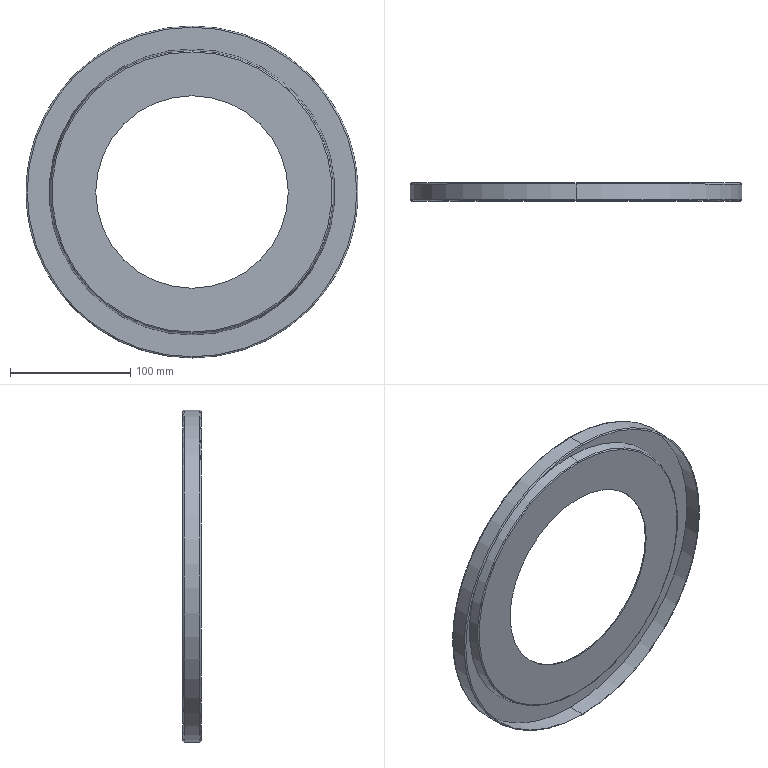Part | SolidWorks | features ICE 2, Fillet 1, Revolution 1 | 1 solid | 25 faces | box 276 x 15 x 276 mm | volume 56604 mm3 | cylinder 8 | torus 8 | plane 5 | cone 4 | commonest cylinder face diameters 160 x2 230 x2 274 x2 276 x2
STEP:
#1=CARTESIAN_POINT('',(0.,-1.,-80.));
#2=VERTEX_POINT('',#1);
#3=CARTESIAN_POINT('',(0.,-1.,80.));
#4=VERTEX_POINT('',#3);
#5=CARTESIAN_POINT('',(0.,-1.,0.));
#6=DIRECTION('',(0.,1.,0.));
#7=DIRECTION('',(0.,0.,1.));
#8=AXIS2_PLACEMENT_3D('',#5,#6,#7);
#9=CIRCLE('',#8,80.);
#10=EDGE_CURVE('',#2,#4,#9,.T.);
#11=ORIENTED_EDGE('',*,*,#10,.F.);
#12=CARTESIAN_POINT('',(0.,-0.01,-80.));
#13=VERTEX_POINT('',#12);
#14=CARTESIAN_POINT('',(0.,-6.,-80.));
#15=DIRECTION('',(0.,1.,0.));
#16=VECTOR('',#15,1000.);
#17=LINE('',#14,#16);
#18=EDGE_CURVE('',#2,#13,#17,.T.);
#19=ORIENTED_EDGE('',*,*,#18,.T.);
#20=CARTESIAN_POINT('',(0.,-0.01,80.));
#21=VERTEX_POINT('',#20);
#22=CARTESIAN_POINT('',(0.,-0.01,0.));
#23=DIRECTION('',(0.,1.,0.));
#24=DIRECTION('',(0.,0.,1.));
#25=AXIS2_PLACEMENT_3D('',#22,#23,#24);
#26=CIRCLE('',#25,80.);
#27=EDGE_CURVE('',#13,#21,#26,.T.);
#28=ORIENTED_EDGE('',*,*,#27,.T.);
#29=CARTESIAN_POINT('',(0.,-6.,80.));
#30=DIRECTION('',(0.,1.,0.));
#31=VECTOR('',#30,1000.);
#32=LINE('',#29,#31);
#33=EDGE_CURVE('',#4,#21,#32,.T.);
#34=ORIENTED_EDGE('',*,*,#33,.F.);
#35=EDGE_LOOP('',(#11,#19,#28,#34));
#36=FACE_OUTER_BOUND('',#35,.T.);
#37=CARTESIAN_POINT('',(0.,-6.,0.));
#38=DIRECTION('',(0.,1.,0.));
#39=DIRECTION('',(0.,0.,1.));
#40=AXIS2_PLACEMENT_3D('',#37,#38,#39);
#41=CYLINDRICAL_SURFACE('',#40,80.);
#42=ADVANCED_FACE('',(#36),#41,.F.);
#43=CARTESIAN_POINT('',(0.,9.,137.));
#44=VERTEX_POINT('',#43);
#45=CARTESIAN_POINT('',(0.,9.,-137.));
#46=VERTEX_POINT('',#45);
#47=CARTESIAN_POINT('',(0.,9.,0.));
#48=DIRECTION('',(0.,1.,0.));
#49=DIRECTION('',(0.,0.,-1.));
#50=AXIS2_PLACEMENT_3D('',#47,#48,#49);
#51=CIRCLE('',#50,137.);
#52=EDGE_CURVE('',#44,#46,#51,.T.);
#53=ORIENTED_EDGE('',*,*,#52,.F.);
#54=CARTESIAN_POINT('',(0.,8.,138.));
#55=VERTEX_POINT('',#54);
#56=CARTESIAN_POINT('',(0.,8.,137.));
#57=DIRECTION('',(1.,0.,0.));
#58=DIRECTION('',(0.,0.,-1.));
#59=AXIS2_PLACEMENT_3D('',#56,#57,#58);
#60=CIRCLE('',#59,1.);
#61=EDGE_CURVE('',#44,#55,#60,.T.);
#62=ORIENTED_EDGE('',*,*,#61,.T.);
#63=CARTESIAN_POINT('',(0.,8.,-138.));
#64=VERTEX_POINT('',#63);
#65=CARTESIAN_POINT('',(0.,8.,0.));
#66=DIRECTION('',(0.,-1.,0.));
#67=DIRECTION('',(0.,0.,-1.));
#68=AXIS2_PLACEMENT_3D('',#65,#66,#67);
#69=CIRCLE('',#68,138.);
#70=EDGE_CURVE('',#64,#55,#69,.T.);
#71=ORIENTED_EDGE('',*,*,#70,.F.);
#72=CARTESIAN_POINT('',(0.,8.,-137.));
#73=DIRECTION('',(-1.,0.,0.));
#74=DIRECTION('',(0.,0.,1.));
#75=AXIS2_PLACEMENT_3D('',#72,#73,#74);
#76=CIRCLE('',#75,1.);
#77=EDGE_CURVE('',#46,#64,#76,.T.);
#78=ORIENTED_EDGE('',*,*,#77,.F.);
#79=EDGE_LOOP('',(#53,#62,#71,#78));
#80=FACE_OUTER_BOUND('',#79,.T.);
#81=CARTESIAN_POINT('',(0.,8.,0.));
#82=DIRECTION('',(0.,-1.,0.));
#83=DIRECTION('',(0.,0.,-1.));
#84=AXIS2_PLACEMENT_3D('',#81,#82,#83);
#85=TOROIDAL_SURFACE('',#84,137.,1.);
#86=ADVANCED_FACE('',(#80),#85,.T.);
#87=CARTESIAN_POINT('',(0.,8.174,117.854));
#88=VERTEX_POINT('',#87);
#89=CARTESIAN_POINT('',(0.,8.174,-117.854));
#90=VERTEX_POINT('',#89);
#91=CARTESIAN_POINT('',(0.,8.174,0.));
#92=DIRECTION('',(0.,1.,0.));
#93=DIRECTION('',(0.,0.,-1.));
#94=AXIS2_PLACEMENT_3D('',#91,#92,#93);
#95=CIRCLE('',#94,117.854);
#96=EDGE_CURVE('',#88,#90,#95,.T.);
#97=ORIENTED_EDGE('',*,*,#96,.F.);
#98=CARTESIAN_POINT('',(0.,9.,118.839));
#99=VERTEX_POINT('',#98);
#100=CARTESIAN_POINT('',(0.,8.,118.839));
#101=DIRECTION('',(1.,0.,0.));
#102=DIRECTION('',(0.,0.,-1.));
#103=AXIS2_PLACEMENT_3D('',#100,#101,#102);
#104=CIRCLE('',#103,1.);
#105=EDGE_CURVE('',#88,#99,#104,.T.);
#106=ORIENTED_EDGE('',*,*,#105,.T.);
#107=CARTESIAN_POINT('',(0.,9.,-118.839));
#108=VERTEX_POINT('',#107);
#109=CARTESIAN_POINT('',(0.,9.,0.));
#110=DIRECTION('',(0.,-1.,0.));
#111=DIRECTION('',(0.,0.,-1.));
#112=AXIS2_PLACEMENT_3D('',#109,#110,#111);
#113=CIRCLE('',#112,118.839);
#114=EDGE_CURVE('',#108,#99,#113,.T.);
#115=ORIENTED_EDGE('',*,*,#114,.F.);
#116=CARTESIAN_POINT('',(0.,8.,-118.839));
#117=DIRECTION('',(-1.,0.,0.));
#118=DIRECTION('',(0.,0.,1.));
#119=AXIS2_PLACEMENT_3D('',#116,#117,#118);
#120=CIRCLE('',#119,1.);
#121=EDGE_CURVE('',#90,#108,#120,.T.);
#122=ORIENTED_EDGE('',*,*,#121,.F.);
#123=EDGE_LOOP('',(#97,#106,#115,#122));
#124=FACE_OUTER_BOUND('',#123,.T.);
#125=CARTESIAN_POINT('',(0.,8.,0.));
#126=DIRECTION('',(0.,-1.,0.));
#127=DIRECTION('',(0.,0.,-1.));
#128=AXIS2_PLACEMENT_3D('',#125,#126,#127);
#129=TOROIDAL_SURFACE('',#128,118.839,1.);
#130=ADVANCED_FACE('',(#124),#129,.T.);
#131=CARTESIAN_POINT('',(0.,-6.,-137.));
#132=VERTEX_POINT('',#131);
#133=CARTESIAN_POINT('',(0.,-6.,137.));
#134=VERTEX_POINT('',#133);
#135=CARTESIAN_POINT('',(0.,-6.,0.));
#136=DIRECTION('',(0.,-1.,0.));
#137=DIRECTION('',(0.,0.,-1.));
#138=AXIS2_PLACEMENT_3D('',#135,#136,#137);
#139=CIRCLE('',#138,137.);
#140=EDGE_CURVE('',#132,#134,#139,.T.);
#141=ORIENTED_EDGE('',*,*,#140,.F.);
#142=CARTESIAN_POINT('',(0.,-5.,-138.));
#143=VERTEX_POINT('',#142);
#144=CARTESIAN_POINT('',(0.,-5.,-137.));
#145=DIRECTION('',(1.,0.,0.));
#146=DIRECTION('',(0.,0.,-1.));
#147=AXIS2_PLACEMENT_3D('',#144,#145,#146);
#148=CIRCLE('',#147,1.);
#149=EDGE_CURVE('',#132,#143,#148,.T.);
#150=ORIENTED_EDGE('',*,*,#149,.T.);
#151=CARTESIAN_POINT('',(0.,-5.,138.));
#152=VERTEX_POINT('',#151);
#153=CARTESIAN_POINT('',(0.,-5.,0.));
#154=DIRECTION('',(0.,1.,0.));
#155=DIRECTION('',(0.,0.,1.));
#156=AXIS2_PLACEMENT_3D('',#153,#154,#155);
#157=CIRCLE('',#156,138.);
#158=EDGE_CURVE('',#152,#143,#157,.T.);
#159=ORIENTED_EDGE('',*,*,#158,.F.);
#160=CARTESIAN_POINT('',(0.,-5.,137.));
#161=DIRECTION('',(-1.,0.,0.));
#162=DIRECTION('',(0.,0.,1.));
#163=AXIS2_PLACEMENT_3D('',#160,#161,#162);
#164=CIRCLE('',#163,1.);
#165=EDGE_CURVE('',#134,#152,#164,.T.);
#166=ORIENTED_EDGE('',*,*,#165,.F.);
#167=EDGE_LOOP('',(#141,#150,#159,#166));
#168=FACE_OUTER_BOUND('',#167,.T.);
#169=CARTESIAN_POINT('',(0.,-5.,0.));
#170=DIRECTION('',(0.,1.,0.));
#171=DIRECTION('',(0.,0.,1.));
#172=AXIS2_PLACEMENT_3D('',#169,#170,#171);
#173=TOROIDAL_SURFACE('',#172,137.,1.);
#174=ADVANCED_FACE('',(#168),#173,.T.);
#175=CARTESIAN_POINT('',(0.,-1.,-116.413));
#176=VERTEX_POINT('',#175);
#177=CARTESIAN_POINT('',(0.,-1.,116.413));
#178=VERTEX_POINT('',#177);
#179=CARTESIAN_POINT('',(0.,-1.,0.));
#180=DIRECTION('',(0.,-1.,0.));
#181=DIRECTION('',(0.,0.,1.));
#182=AXIS2_PLACEMENT_3D('',#179,#180,#181);
#183=CIRCLE('',#182,116.413);
#184=EDGE_CURVE('',#176,#178,#183,.T.);
#185=ORIENTED_EDGE('',*,*,#184,.F.);
#186=CARTESIAN_POINT('',(0.,-0.1736,-117.398));
#187=VERTEX_POINT('',#186);
#188=CARTESIAN_POINT('',(0.,0.,-116.413));
#189=DIRECTION('',(1.,0.,0.));
#190=DIRECTION('',(0.,0.,-1.));
#191=AXIS2_PLACEMENT_3D('',#188,#189,#190);
#192=CIRCLE('',#191,1.);
#193=EDGE_CURVE('',#176,#187,#192,.T.);
#194=ORIENTED_EDGE('',*,*,#193,.T.);
#195=CARTESIAN_POINT('',(0.,-0.1736,117.398));
#196=VERTEX_POINT('',#195);
#197=CARTESIAN_POINT('',(0.,-0.1736,0.));
#198=DIRECTION('',(0.,1.,0.));
#199=DIRECTION('',(0.,0.,-1.));
#200=AXIS2_PLACEMENT_3D('',#197,#198,#199);
#201=CIRCLE('',#200,117.398);
#202=EDGE_CURVE('',#196,#187,#201,.T.);
#203=ORIENTED_EDGE('',*,*,#202,.F.);
#204=CARTESIAN_POINT('',(0.,0.,116.413));
#205=DIRECTION('',(-1.,0.,0.));
#206=DIRECTION('',(0.,0.,1.));
#207=AXIS2_PLACEMENT_3D('',#204,#205,#206);
#208=CIRCLE('',#207,1.);
#209=EDGE_CURVE('',#178,#196,#208,.T.);
#210=ORIENTED_EDGE('',*,*,#209,.F.);
#211=EDGE_LOOP('',(#185,#194,#203,#210));
#212=FACE_OUTER_BOUND('',#211,.T.);
#213=CARTESIAN_POINT('',(0.,0.,0.));
#214=DIRECTION('',(0.,1.,0.));
#215=DIRECTION('',(0.,0.,1.));
#216=AXIS2_PLACEMENT_3D('',#213,#214,#215);
#217=TOROIDAL_SURFACE('',#216,116.413,1.);
#218=ADVANCED_FACE('',(#212),#217,.T.);
#219=CARTESIAN_POINT('',(0.,-0.01,-115.));
#220=VERTEX_POINT('',#219);
#221=CARTESIAN_POINT('',(0.,-0.01,115.));
#222=VERTEX_POINT('',#221);
#223=CARTESIAN_POINT('',(0.,-0.01,0.));
#224=DIRECTION('',(0.,1.,0.));
#225=DIRECTION('',(0.,0.,1.));
#226=AXIS2_PLACEMENT_3D('',#223,#224,#225);
#227=CIRCLE('',#226,115.);
#228=EDGE_CURVE('',#220,#222,#227,.T.);
#229=ORIENTED_EDGE('',*,*,#228,.F.);
#230=CARTESIAN_POINT('',(0.,0.,-115.));
#231=VERTEX_POINT('',#230);
#232=CARTESIAN_POINT('',(0.,-0.01,-115.));
#233=DIRECTION('',(0.,1.,0.));
#234=VECTOR('',#233,1000.);
#235=LINE('',#232,#234);
#236=EDGE_CURVE('',#220,#231,#235,.T.);
#237=ORIENTED_EDGE('',*,*,#236,.T.);
#238=CARTESIAN_POINT('',(0.,0.,115.));
#239=VERTEX_POINT('',#238);
#240=CARTESIAN_POINT('',(0.,0.,0.));
#241=DIRECTION('',(0.,1.,0.));
#242=DIRECTION('',(0.,0.,1.));
#243=AXIS2_PLACEMENT_3D('',#240,#241,#242);
#244=CIRCLE('',#243,115.);
#245=EDGE_CURVE('',#231,#239,#244,.T.);
#246=ORIENTED_EDGE('',*,*,#245,.T.);
#247=CARTESIAN_POINT('',(0.,-0.01,115.));
#248=DIRECTION('',(0.,1.,0.));
#249=VECTOR('',#248,1000.);
#250=LINE('',#247,#249);
#251=EDGE_CURVE('',#222,#239,#250,.T.);
#252=ORIENTED_EDGE('',*,*,#251,.F.);
#253=EDGE_LOOP('',(#229,#237,#246,#252));
#254=FACE_OUTER_BOUND('',#253,.T.);
#255=CARTESIAN_POINT('',(0.,-0.01,0.));
#256=DIRECTION('',(0.,1.,0.));
#257=DIRECTION('',(0.,0.,1.));
#258=AXIS2_PLACEMENT_3D('',#255,#256,#257);
#259=CYLINDRICAL_SURFACE('',#258,115.);
#260=ADVANCED_FACE('',(#254),#259,.F.);
#261=ORIENTED_EDGE('',*,*,#202,.T.);
#262=CARTESIAN_POINT('',(0.,8.,-118.839));
#263=VERTEX_POINT('',#262);
#264=CARTESIAN_POINT('',(0.,8.,-118.839));
#265=DIRECTION('',(0.,0.9848,-0.1736));
#266=VECTOR('',#265,1000.);
#267=LINE('',#264,#266);
#268=EDGE_CURVE('',#187,#263,#267,.T.);
#269=ORIENTED_EDGE('',*,*,#268,.T.);
#270=CARTESIAN_POINT('',(0.,8.,118.839));
#271=VERTEX_POINT('',#270);
#272=CARTESIAN_POINT('',(0.,8.,0.));
#273=DIRECTION('',(0.,-1.,0.));
#274=DIRECTION('',(0.,0.,-1.));
#275=AXIS2_PLACEMENT_3D('',#272,#273,#274);
#276=CIRCLE('',#275,118.839);
#277=EDGE_CURVE('',#263,#271,#276,.T.);
#278=ORIENTED_EDGE('',*,*,#277,.T.);
#279=CARTESIAN_POINT('',(0.,8.,118.839));
#280=DIRECTION('',(0.,0.9848,0.1736));
#281=VECTOR('',#280,1000.);
#282=LINE('',#279,#281);
#283=EDGE_CURVE('',#196,#271,#282,.T.);
#284=ORIENTED_EDGE('',*,*,#283,.F.);
#285=EDGE_LOOP('',(#261,#269,#278,#284));
#286=FACE_OUTER_BOUND('',#285,.T.);
#287=CARTESIAN_POINT('',(0.,8.,0.));
#288=DIRECTION('',(0.,1.,0.));
#289=DIRECTION('',(0.,0.,1.));
#290=AXIS2_PLACEMENT_3D('',#287,#288,#289);
#291=CONICAL_SURFACE('',#290,118.839,0.1745);
#292=ADVANCED_FACE('',(#286),#291,.T.);
#293=CARTESIAN_POINT('',(0.,8.,137.));
#294=VERTEX_POINT('',#293);
#295=CARTESIAN_POINT('',(0.,8.,-137.));
#296=VERTEX_POINT('',#295);
#297=CARTESIAN_POINT('',(0.,8.,0.));
#298=DIRECTION('',(0.,-1.,0.));
#299=DIRECTION('',(0.,0.,-1.));
#300=AXIS2_PLACEMENT_3D('',#297,#298,#299);
#301=CIRCLE('',#300,137.);
#302=EDGE_CURVE('',#294,#296,#301,.T.);
#303=ORIENTED_EDGE('',*,*,#302,.F.);
#304=CARTESIAN_POINT('',(0.,0.,137.));
#305=DIRECTION('',(0.,-1.,0.));
#306=VECTOR('',#305,1000.);
#307=LINE('',#304,#306);
#308=EDGE_CURVE('',#294,#134,#307,.T.);
#309=ORIENTED_EDGE('',*,*,#308,.T.);
#310=CARTESIAN_POINT('',(0.,-6.,0.));
#311=DIRECTION('',(0.,-1.,0.));
#312=DIRECTION('',(0.,0.,-1.));
#313=AXIS2_PLACEMENT_3D('',#310,#311,#312);
#314=CIRCLE('',#313,137.);
#315=EDGE_CURVE('',#134,#132,#314,.T.);
#316=ORIENTED_EDGE('',*,*,#315,.T.);
#317=CARTESIAN_POINT('',(0.,0.,-137.));
#318=DIRECTION('',(0.,-1.,0.));
#319=VECTOR('',#318,1000.);
#320=LINE('',#317,#319);
#321=EDGE_CURVE('',#296,#132,#320,.T.);
#322=ORIENTED_EDGE('',*,*,#321,.F.);
#323=EDGE_LOOP('',(#303,#309,#316,#322));
#324=FACE_OUTER_BOUND('',#323,.T.);
#325=CARTESIAN_POINT('',(0.,0.,0.));
#326=DIRECTION('',(0.,-1.,0.));
#327=DIRECTION('',(0.,0.,-1.));
#328=AXIS2_PLACEMENT_3D('',#325,#326,#327);
#329=CYLINDRICAL_SURFACE('',#328,137.);
#330=ADVANCED_FACE('',(#324),#329,.F.);
#331=ORIENTED_EDGE('',*,*,#70,.T.);
#332=CARTESIAN_POINT('',(0.,0.,138.));
#333=DIRECTION('',(0.,-1.,0.));
#334=VECTOR('',#333,1000.);
#335=LINE('',#332,#334);
#336=EDGE_CURVE('',#55,#152,#335,.T.);
#337=ORIENTED_EDGE('',*,*,#336,.T.);
#338=ORIENTED_EDGE('',*,*,#158,.T.);
#339=CARTESIAN_POINT('',(0.,0.,-138.));
#340=DIRECTION('',(0.,-1.,0.));
#341=VECTOR('',#340,1000.);
#342=LINE('',#339,#341);
#343=EDGE_CURVE('',#64,#143,#342,.T.);
#344=ORIENTED_EDGE('',*,*,#343,.F.);
#345=EDGE_LOOP('',(#331,#337,#338,#344));
#346=FACE_OUTER_BOUND('',#345,.T.);
#347=CARTESIAN_POINT('',(0.,0.,0.));
#348=DIRECTION('',(0.,-1.,0.));
#349=DIRECTION('',(0.,0.,-1.));
#350=AXIS2_PLACEMENT_3D('',#347,#348,#349);
#351=CYLINDRICAL_SURFACE('',#350,138.);
#352=ADVANCED_FACE('',(#346),#351,.T.);
#353=CARTESIAN_POINT('',(0.,0.,116.413));
#354=VERTEX_POINT('',#353);
#355=CARTESIAN_POINT('',(0.,0.,-116.413));
#356=VERTEX_POINT('',#355);
#357=CARTESIAN_POINT('',(0.,0.,0.));
#358=DIRECTION('',(0.,-1.,0.));
#359=DIRECTION('',(0.,0.,-1.));
#360=AXIS2_PLACEMENT_3D('',#357,#358,#359);
#361=CIRCLE('',#360,116.413);
#362=EDGE_CURVE('',#354,#356,#361,.T.);
#363=ORIENTED_EDGE('',*,*,#362,.T.);
#364=CARTESIAN_POINT('',(0.,0.,-116.413));
#365=DIRECTION('',(0.,0.9848,-0.1736));
#366=VECTOR('',#365,1000.);
#367=LINE('',#364,#366);
#368=EDGE_CURVE('',#356,#90,#367,.T.);
#369=ORIENTED_EDGE('',*,*,#368,.T.);
#370=CARTESIAN_POINT('',(0.,8.174,0.));
#371=DIRECTION('',(0.,1.,0.));
#372=DIRECTION('',(0.,0.,-1.));
#373=AXIS2_PLACEMENT_3D('',#370,#371,#372);
#374=CIRCLE('',#373,117.854);
#375=EDGE_CURVE('',#90,#88,#374,.T.);
#376=ORIENTED_EDGE('',*,*,#375,.T.);
#377=CARTESIAN_POINT('',(0.,0.,116.413));
#378=DIRECTION('',(0.,0.9848,0.1736));
#379=VECTOR('',#378,1000.);
#380=LINE('',#377,#379);
#381=EDGE_CURVE('',#354,#88,#380,.T.);
#382=ORIENTED_EDGE('',*,*,#381,.F.);
#383=EDGE_LOOP('',(#363,#369,#376,#382));
#384=FACE_OUTER_BOUND('',#383,.T.);
#385=CARTESIAN_POINT('',(0.,0.,0.));
#386=DIRECTION('',(0.,1.,0.));
#387=DIRECTION('',(0.,0.,1.));
#388=AXIS2_PLACEMENT_3D('',#385,#386,#387);
#389=CONICAL_SURFACE('',#388,116.413,0.1745);
#390=ADVANCED_FACE('',(#384),#389,.F.);
#391=CARTESIAN_POINT('',(0.,0.,0.));
#392=DIRECTION('',(0.,1.,0.));
#393=DIRECTION('',(0.,0.,1.));
#394=AXIS2_PLACEMENT_3D('',#391,#392,#393);
#395=CIRCLE('',#394,115.);
#396=EDGE_CURVE('',#239,#231,#395,.T.);
#397=ORIENTED_EDGE('',*,*,#396,.F.);
#398=ORIENTED_EDGE('',*,*,#245,.F.);
#399=EDGE_LOOP('',(#397,#398));
#400=FACE_BOUND('',#399,.T.);
#401=ORIENTED_EDGE('',*,*,#362,.F.);
#402=CARTESIAN_POINT('',(0.,0.,0.));
#403=DIRECTION('',(0.,-1.,0.));
#404=DIRECTION('',(0.,0.,-1.));
#405=AXIS2_PLACEMENT_3D('',#402,#403,#404);
#406=CIRCLE('',#405,116.413);
#407=EDGE_CURVE('',#356,#354,#406,.T.);
#408=ORIENTED_EDGE('',*,*,#407,.F.);
#409=EDGE_LOOP('',(#401,#408));
#410=FACE_OUTER_BOUND('',#409,.T.);
#411=CARTESIAN_POINT('',(0.,0.,0.));
#412=DIRECTION('',(0.,-1.,0.));
#413=DIRECTION('',(0.,0.,-1.));
#414=AXIS2_PLACEMENT_3D('',#411,#412,#413);
#415=PLANE('',#414);
#416=ADVANCED_FACE('',(#400,#410),#415,.F.);
#417=ORIENTED_EDGE('',*,*,#368,.F.);
#418=ORIENTED_EDGE('',*,*,#407,.T.);
#419=ORIENTED_EDGE('',*,*,#381,.T.);
#420=ORIENTED_EDGE('',*,*,#96,.T.);
#421=EDGE_LOOP('',(#417,#418,#419,#420));
#422=FACE_OUTER_BOUND('',#421,.T.);
#423=CARTESIAN_POINT('',(0.,0.,0.));
#424=DIRECTION('',(0.,1.,0.));
#425=DIRECTION('',(0.,0.,1.));
#426=AXIS2_PLACEMENT_3D('',#423,#424,#425);
#427=CONICAL_SURFACE('',#426,116.413,0.1745);
#428=ADVANCED_FACE('',(#422),#427,.F.);
#429=ORIENTED_EDGE('',*,*,#114,.T.);
#430=CARTESIAN_POINT('',(0.,9.,0.));
#431=DIRECTION('',(0.,-1.,0.));
#432=DIRECTION('',(0.,0.,-1.));
#433=AXIS2_PLACEMENT_3D('',#430,#431,#432);
#434=CIRCLE('',#433,118.839);
#435=EDGE_CURVE('',#99,#108,#434,.T.);
#436=ORIENTED_EDGE('',*,*,#435,.T.);
#437=EDGE_LOOP('',(#429,#436));
#438=FACE_BOUND('',#437,.T.);
#439=CARTESIAN_POINT('',(0.,9.,0.));
#440=DIRECTION('',(0.,1.,0.));
#441=DIRECTION('',(0.,0.,-1.));
#442=AXIS2_PLACEMENT_3D('',#439,#440,#441);
#443=CIRCLE('',#442,137.);
#444=EDGE_CURVE('',#46,#44,#443,.T.);
#445=ORIENTED_EDGE('',*,*,#444,.T.);
#446=ORIENTED_EDGE('',*,*,#52,.T.);
#447=EDGE_LOOP('',(#445,#446));
#448=FACE_OUTER_BOUND('',#447,.T.);
#449=CARTESIAN_POINT('',(-118.,9.,0.));
#450=DIRECTION('',(0.,-1.,0.));
#451=DIRECTION('',(0.,0.,-1.));
#452=AXIS2_PLACEMENT_3D('',#449,#450,#451);
#453=PLANE('',#452);
#454=ADVANCED_FACE('',(#438,#448),#453,.F.);
#455=ORIENTED_EDGE('',*,*,#336,.F.);
#456=CARTESIAN_POINT('',(0.,8.,0.));
#457=DIRECTION('',(0.,-1.,0.));
#458=DIRECTION('',(0.,0.,-1.));
#459=AXIS2_PLACEMENT_3D('',#456,#457,#458);
#460=CIRCLE('',#459,138.);
#461=EDGE_CURVE('',#55,#64,#460,.T.);
#462=ORIENTED_EDGE('',*,*,#461,.T.);
#463=ORIENTED_EDGE('',*,*,#343,.T.);
#464=CARTESIAN_POINT('',(0.,-5.,0.));
#465=DIRECTION('',(0.,1.,0.));
#466=DIRECTION('',(0.,0.,1.));
#467=AXIS2_PLACEMENT_3D('',#464,#465,#466);
#468=CIRCLE('',#467,138.);
#469=EDGE_CURVE('',#143,#152,#468,.T.);
#470=ORIENTED_EDGE('',*,*,#469,.T.);
#471=EDGE_LOOP('',(#455,#462,#463,#470));
#472=FACE_OUTER_BOUND('',#471,.T.);
#473=CARTESIAN_POINT('',(0.,0.,0.));
#474=DIRECTION('',(0.,-1.,0.));
#475=DIRECTION('',(0.,0.,-1.));
#476=AXIS2_PLACEMENT_3D('',#473,#474,#475);
#477=CYLINDRICAL_SURFACE('',#476,138.);
#478=ADVANCED_FACE('',(#472),#477,.T.);
#479=ORIENTED_EDGE('',*,*,#308,.F.);
#480=CARTESIAN_POINT('',(0.,8.,0.));
#481=DIRECTION('',(0.,-1.,0.));
#482=DIRECTION('',(0.,0.,-1.));
#483=AXIS2_PLACEMENT_3D('',#480,#481,#482);
#484=CIRCLE('',#483,137.);
#485=EDGE_CURVE('',#296,#294,#484,.T.);
#486=ORIENTED_EDGE('',*,*,#485,.F.);
#487=ORIENTED_EDGE('',*,*,#321,.T.);
#488=ORIENTED_EDGE('',*,*,#140,.T.);
#489=EDGE_LOOP('',(#479,#486,#487,#488));
#490=FACE_OUTER_BOUND('',#489,.T.);
#491=CARTESIAN_POINT('',(0.,0.,0.));
#492=DIRECTION('',(0.,-1.,0.));
#493=DIRECTION('',(0.,0.,-1.));
#494=AXIS2_PLACEMENT_3D('',#491,#492,#493);
#495=CYLINDRICAL_SURFACE('',#494,137.);
#496=ADVANCED_FACE('',(#490),#495,.F.);
#497=CARTESIAN_POINT('',(0.,8.,0.));
#498=DIRECTION('',(0.,-1.,0.));
#499=DIRECTION('',(0.,0.,-1.));
#500=AXIS2_PLACEMENT_3D('',#497,#498,#499);
#501=CIRCLE('',#500,118.839);
#502=EDGE_CURVE('',#271,#263,#501,.T.);
#503=ORIENTED_EDGE('',*,*,#502,.F.);
#504=ORIENTED_EDGE('',*,*,#277,.F.);
#505=EDGE_LOOP('',(#503,#504));
#506=FACE_BOUND('',#505,.T.);
#507=ORIENTED_EDGE('',*,*,#485,.T.);
#508=ORIENTED_EDGE('',*,*,#302,.T.);
#509=EDGE_LOOP('',(#507,#508));
#510=FACE_OUTER_BOUND('',#509,.T.);
#511=CARTESIAN_POINT('',(-137.,8.,0.));
#512=DIRECTION('',(0.,1.,0.));
#513=DIRECTION('',(0.,0.,1.));
#514=AXIS2_PLACEMENT_3D('',#511,#512,#513);
#515=PLANE('',#514);
#516=ADVANCED_FACE('',(#506,#510),#515,.F.);
#517=ORIENTED_EDGE('',*,*,#268,.F.);
#518=CARTESIAN_POINT('',(0.,-0.1736,0.));
#519=DIRECTION('',(0.,1.,0.));
#520=DIRECTION('',(0.,0.,-1.));
#521=AXIS2_PLACEMENT_3D('',#518,#519,#520);
#522=CIRCLE('',#521,117.398);
#523=EDGE_CURVE('',#187,#196,#522,.T.);
#524=ORIENTED_EDGE('',*,*,#523,.T.);
#525=ORIENTED_EDGE('',*,*,#283,.T.);
#526=ORIENTED_EDGE('',*,*,#502,.T.);
#527=EDGE_LOOP('',(#517,#524,#525,#526));
#528=FACE_OUTER_BOUND('',#527,.T.);
#529=CARTESIAN_POINT('',(0.,8.,0.));
#530=DIRECTION('',(0.,1.,0.));
#531=DIRECTION('',(0.,0.,1.));
#532=AXIS2_PLACEMENT_3D('',#529,#530,#531);
#533=CONICAL_SURFACE('',#532,118.839,0.1745);
#534=ADVANCED_FACE('',(#528),#533,.T.);
#535=CARTESIAN_POINT('',(0.,-1.,0.));
#536=DIRECTION('',(0.,1.,0.));
#537=DIRECTION('',(0.,0.,1.));
#538=AXIS2_PLACEMENT_3D('',#535,#536,#537);
#539=CIRCLE('',#538,80.);
#540=EDGE_CURVE('',#4,#2,#539,.T.);
#541=ORIENTED_EDGE('',*,*,#540,.T.);
#542=ORIENTED_EDGE('',*,*,#10,.T.);
#543=EDGE_LOOP('',(#541,#542));
#544=FACE_BOUND('',#543,.T.);
#545=CARTESIAN_POINT('',(0.,-1.,0.));
#546=DIRECTION('',(0.,-1.,0.));
#547=DIRECTION('',(0.,0.,1.));
#548=AXIS2_PLACEMENT_3D('',#545,#546,#547);
#549=CIRCLE('',#548,116.413);
#550=EDGE_CURVE('',#178,#176,#549,.T.);
#551=ORIENTED_EDGE('',*,*,#550,.T.);
#552=ORIENTED_EDGE('',*,*,#184,.T.);
#553=EDGE_LOOP('',(#551,#552));
#554=FACE_OUTER_BOUND('',#553,.T.);
#555=CARTESIAN_POINT('',(-117.252,-1.,0.));
#556=DIRECTION('',(0.,1.,0.));
#557=DIRECTION('',(0.,0.,1.));
#558=AXIS2_PLACEMENT_3D('',#555,#556,#557);
#559=PLANE('',#558);
#560=ADVANCED_FACE('',(#544,#554),#559,.F.);
#561=ORIENTED_EDGE('',*,*,#236,.F.);
#562=CARTESIAN_POINT('',(0.,-0.01,0.));
#563=DIRECTION('',(0.,1.,0.));
#564=DIRECTION('',(0.,0.,1.));
#565=AXIS2_PLACEMENT_3D('',#562,#563,#564);
#566=CIRCLE('',#565,115.);
#567=EDGE_CURVE('',#222,#220,#566,.T.);
#568=ORIENTED_EDGE('',*,*,#567,.F.);
#569=ORIENTED_EDGE('',*,*,#251,.T.);
#570=ORIENTED_EDGE('',*,*,#396,.T.);
#571=EDGE_LOOP('',(#561,#568,#569,#570));
#572=FACE_OUTER_BOUND('',#571,.T.);
#573=CARTESIAN_POINT('',(0.,-0.01,0.));
#574=DIRECTION('',(0.,1.,0.));
#575=DIRECTION('',(0.,0.,1.));
#576=AXIS2_PLACEMENT_3D('',#573,#574,#575);
#577=CYLINDRICAL_SURFACE('',#576,115.);
#578=ADVANCED_FACE('',(#572),#577,.F.);
#579=CARTESIAN_POINT('',(0.,-0.01,0.));
#580=DIRECTION('',(0.,1.,0.));
#581=DIRECTION('',(0.,0.,1.));
#582=AXIS2_PLACEMENT_3D('',#579,#580,#581);
#583=CIRCLE('',#582,80.);
#584=EDGE_CURVE('',#21,#13,#583,.T.);
#585=ORIENTED_EDGE('',*,*,#584,.F.);
#586=ORIENTED_EDGE('',*,*,#27,.F.);
#587=EDGE_LOOP('',(#585,#586));
#588=FACE_BOUND('',#587,.T.);
#589=ORIENTED_EDGE('',*,*,#567,.T.);
#590=ORIENTED_EDGE('',*,*,#228,.T.);
#591=EDGE_LOOP('',(#589,#590));
#592=FACE_OUTER_BOUND('',#591,.T.);
#593=CARTESIAN_POINT('',(0.,-0.01,0.));
#594=DIRECTION('',(0.,1.,0.));
#595=DIRECTION('',(0.,0.,1.));
#596=AXIS2_PLACEMENT_3D('',#593,#594,#595);
#597=PLANE('',#596);
#598=ADVANCED_FACE('',(#588,#592),#597,.T.);
#599=ORIENTED_EDGE('',*,*,#193,.F.);
#600=ORIENTED_EDGE('',*,*,#550,.F.);
#601=ORIENTED_EDGE('',*,*,#209,.T.);
#602=ORIENTED_EDGE('',*,*,#523,.F.);
#603=EDGE_LOOP('',(#599,#600,#601,#602));
#604=FACE_OUTER_BOUND('',#603,.T.);
#605=CARTESIAN_POINT('',(0.,0.,0.));
#606=DIRECTION('',(0.,1.,0.));
#607=DIRECTION('',(0.,0.,1.));
#608=AXIS2_PLACEMENT_3D('',#605,#606,#607);
#609=TOROIDAL_SURFACE('',#608,116.413,1.);
#610=ADVANCED_FACE('',(#604),#609,.T.);
#611=ORIENTED_EDGE('',*,*,#149,.F.);
#612=ORIENTED_EDGE('',*,*,#315,.F.);
#613=ORIENTED_EDGE('',*,*,#165,.T.);
#614=ORIENTED_EDGE('',*,*,#469,.F.);
#615=EDGE_LOOP('',(#611,#612,#613,#614));
#616=FACE_OUTER_BOUND('',#615,.T.);
#617=CARTESIAN_POINT('',(0.,-5.,0.));
#618=DIRECTION('',(0.,1.,0.));
#619=DIRECTION('',(0.,0.,1.));
#620=AXIS2_PLACEMENT_3D('',#617,#618,#619);
#621=TOROIDAL_SURFACE('',#620,137.,1.);
#622=ADVANCED_FACE('',(#616),#621,.T.);
#623=ORIENTED_EDGE('',*,*,#105,.F.);
#624=ORIENTED_EDGE('',*,*,#375,.F.);
#625=ORIENTED_EDGE('',*,*,#121,.T.);
#626=ORIENTED_EDGE('',*,*,#435,.F.);
#627=EDGE_LOOP('',(#623,#624,#625,#626));
#628=FACE_OUTER_BOUND('',#627,.T.);
#629=CARTESIAN_POINT('',(0.,8.,0.));
#630=DIRECTION('',(0.,-1.,0.));
#631=DIRECTION('',(0.,0.,-1.));
#632=AXIS2_PLACEMENT_3D('',#629,#630,#631);
#633=TOROIDAL_SURFACE('',#632,118.839,1.);
#634=ADVANCED_FACE('',(#628),#633,.T.);
#635=ORIENTED_EDGE('',*,*,#61,.F.);
#636=ORIENTED_EDGE('',*,*,#444,.F.);
#637=ORIENTED_EDGE('',*,*,#77,.T.);
#638=ORIENTED_EDGE('',*,*,#461,.F.);
#639=EDGE_LOOP('',(#635,#636,#637,#638));
#640=FACE_OUTER_BOUND('',#639,.T.);
#641=CARTESIAN_POINT('',(0.,8.,0.));
#642=DIRECTION('',(0.,-1.,0.));
#643=DIRECTION('',(0.,0.,-1.));
#644=AXIS2_PLACEMENT_3D('',#641,#642,#643);
#645=TOROIDAL_SURFACE('',#644,137.,1.);
#646=ADVANCED_FACE('',(#640),#645,.T.);
#647=ORIENTED_EDGE('',*,*,#18,.F.);
#648=ORIENTED_EDGE('',*,*,#540,.F.);
#649=ORIENTED_EDGE('',*,*,#33,.T.);
#650=ORIENTED_EDGE('',*,*,#584,.T.);
#651=EDGE_LOOP('',(#647,#648,#649,#650));
#652=FACE_OUTER_BOUND('',#651,.T.);
#653=CARTESIAN_POINT('',(0.,-6.,0.));
#654=DIRECTION('',(0.,1.,0.));
#655=DIRECTION('',(0.,0.,1.));
#656=AXIS2_PLACEMENT_3D('',#653,#654,#655);
#657=CYLINDRICAL_SURFACE('',#656,80.);
#658=ADVANCED_FACE('',(#652),#657,.F.);
#659=CLOSED_SHELL('',(#42,#86,#130,#174,#218,#260,#292,#330,#352,#390,#416,#428,#454,#478,#496,#516,#534,#560,#578,#598,#610,#622,#634,#646,#658));
#660=MANIFOLD_SOLID_BREP('',#659);
#661=CARTESIAN_POINT('',(0.,0.,0.));
#662=DIRECTION('',(0.,0.,1.));
#663=DIRECTION('',(1.,0.,0.));
#664=AXIS2_PLACEMENT_3D('',#661,#662,#663);
#665=(LENGTH_UNIT()NAMED_UNIT(*)SI_UNIT(.MILLI.,.METRE.));
#666=UNCERTAINTY_MEASURE_WITH_UNIT(LENGTH_MEASURE(0.00001),#665,'','');
#667=(NAMED_UNIT(*)PLANE_ANGLE_UNIT()SI_UNIT($,.RADIAN.));
#668=(NAMED_UNIT(*)SI_UNIT($,.STERADIAN.)SOLID_ANGLE_UNIT());
#669=(GEOMETRIC_REPRESENTATION_CONTEXT(3)GLOBAL_UNCERTAINTY_ASSIGNED_CONTEXT((#666))GLOBAL_UNIT_ASSIGNED_CONTEXT((#665,#667,#668))REPRESENTATION_CONTEXT('',''));
#670=ADVANCED_BREP_SHAPE_REPRESENTATION('',(#660,#664),#669);